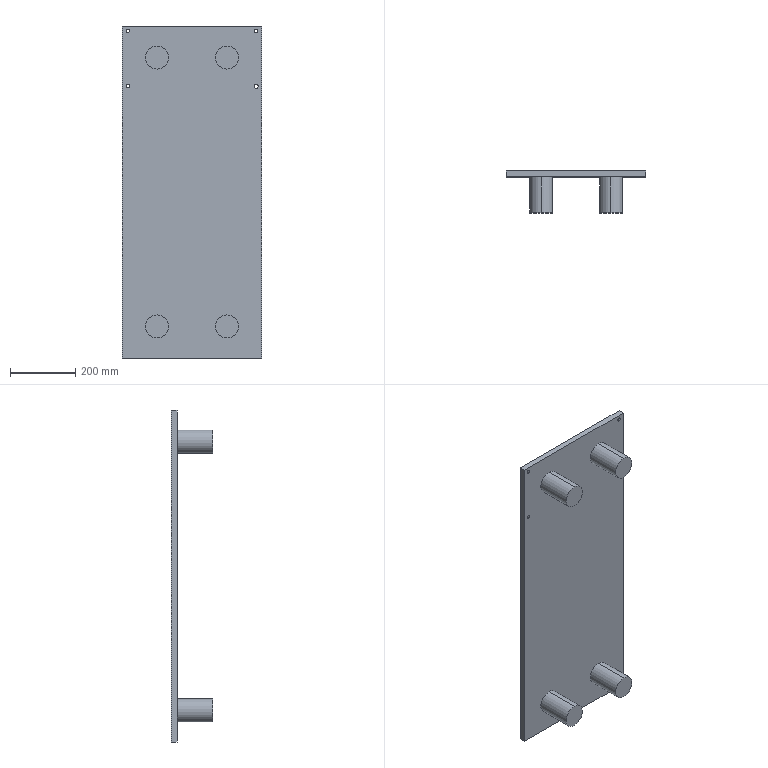Part | SolidWorks | features Extrusion 1, ICE 1 | 1 solid | 26 faces | box 430 x 128 x 1020 mm | volume 9620878 mm3 | cylinder 16 | plane 10 | commonest cylinder face diameters 70.779 x8 10.158 x2 10.702 x2 11 x2 12.721 x2
STEP:
#1=CARTESIAN_POINT('',(96.666,-110.,-468.564));
#2=VERTEX_POINT('',#1);
#3=CARTESIAN_POINT('',(96.666,-110.,-397.785));
#4=VERTEX_POINT('',#3);
#5=CARTESIAN_POINT('',(96.666,-110.,-433.174));
#6=DIRECTION('',(0.,-1.,0.));
#7=DIRECTION('',(0.,0.,1.));
#8=AXIS2_PLACEMENT_3D('',#5,#6,#7);
#9=CIRCLE('',#8,35.39);
#10=EDGE_CURVE('',#2,#4,#9,.T.);
#11=ORIENTED_EDGE('',*,*,#10,.F.);
#12=CARTESIAN_POINT('',(96.666,0.,-468.564));
#13=VERTEX_POINT('',#12);
#14=CARTESIAN_POINT('',(96.666,-110.,-468.564));
#15=DIRECTION('',(0.,1.,0.));
#16=VECTOR('',#15,1000.);
#17=LINE('',#14,#16);
#18=EDGE_CURVE('',#2,#13,#17,.T.);
#19=ORIENTED_EDGE('',*,*,#18,.T.);
#20=CARTESIAN_POINT('',(96.666,0.,-397.785));
#21=VERTEX_POINT('',#20);
#22=CARTESIAN_POINT('',(96.666,0.,-433.174));
#23=DIRECTION('',(0.,-1.,0.));
#24=DIRECTION('',(0.,0.,1.));
#25=AXIS2_PLACEMENT_3D('',#22,#23,#24);
#26=CIRCLE('',#25,35.39);
#27=EDGE_CURVE('',#13,#21,#26,.T.);
#28=ORIENTED_EDGE('',*,*,#27,.T.);
#29=CARTESIAN_POINT('',(96.666,-110.,-397.785));
#30=DIRECTION('',(0.,1.,0.));
#31=VECTOR('',#30,1000.);
#32=LINE('',#29,#31);
#33=EDGE_CURVE('',#4,#21,#32,.T.);
#34=ORIENTED_EDGE('',*,*,#33,.F.);
#35=EDGE_LOOP('',(#11,#19,#28,#34));
#36=FACE_OUTER_BOUND('',#35,.T.);
#37=CARTESIAN_POINT('',(96.666,-110.,-433.174));
#38=DIRECTION('',(0.,1.,0.));
#39=DIRECTION('',(0.,0.,1.));
#40=AXIS2_PLACEMENT_3D('',#37,#38,#39);
#41=CYLINDRICAL_SURFACE('',#40,35.39);
#42=ADVANCED_FACE('',(#36),#41,.T.);
#43=CARTESIAN_POINT('',(-118.27,-110.,-468.564));
#44=VERTEX_POINT('',#43);
#45=CARTESIAN_POINT('',(-118.27,-110.,-397.785));
#46=VERTEX_POINT('',#45);
#47=CARTESIAN_POINT('',(-118.27,-110.,-433.174));
#48=DIRECTION('',(0.,-1.,0.));
#49=DIRECTION('',(0.,0.,-1.));
#50=AXIS2_PLACEMENT_3D('',#47,#48,#49);
#51=CIRCLE('',#50,35.39);
#52=EDGE_CURVE('',#44,#46,#51,.T.);
#53=ORIENTED_EDGE('',*,*,#52,.F.);
#54=CARTESIAN_POINT('',(-118.27,0.,-468.564));
#55=VERTEX_POINT('',#54);
#56=CARTESIAN_POINT('',(-118.27,-110.,-468.564));
#57=DIRECTION('',(0.,1.,0.));
#58=VECTOR('',#57,1000.);
#59=LINE('',#56,#58);
#60=EDGE_CURVE('',#44,#55,#59,.T.);
#61=ORIENTED_EDGE('',*,*,#60,.T.);
#62=CARTESIAN_POINT('',(-118.27,0.,-397.785));
#63=VERTEX_POINT('',#62);
#64=CARTESIAN_POINT('',(-118.27,0.,-433.174));
#65=DIRECTION('',(0.,-1.,0.));
#66=DIRECTION('',(0.,0.,1.));
#67=AXIS2_PLACEMENT_3D('',#64,#65,#66);
#68=CIRCLE('',#67,35.39);
#69=EDGE_CURVE('',#55,#63,#68,.T.);
#70=ORIENTED_EDGE('',*,*,#69,.T.);
#71=CARTESIAN_POINT('',(-118.27,-110.,-397.785));
#72=DIRECTION('',(0.,1.,0.));
#73=VECTOR('',#72,1000.);
#74=LINE('',#71,#73);
#75=EDGE_CURVE('',#46,#63,#74,.T.);
#76=ORIENTED_EDGE('',*,*,#75,.F.);
#77=EDGE_LOOP('',(#53,#61,#70,#76));
#78=FACE_OUTER_BOUND('',#77,.T.);
#79=CARTESIAN_POINT('',(-118.27,-110.,-433.174));
#80=DIRECTION('',(0.,1.,0.));
#81=DIRECTION('',(0.,0.,1.));
#82=AXIS2_PLACEMENT_3D('',#79,#80,#81);
#83=CYLINDRICAL_SURFACE('',#82,35.39);
#84=ADVANCED_FACE('',(#78),#83,.T.);
#85=CARTESIAN_POINT('',(-118.27,-110.,357.683));
#86=VERTEX_POINT('',#85);
#87=CARTESIAN_POINT('',(-118.27,-110.,428.463));
#88=VERTEX_POINT('',#87);
#89=CARTESIAN_POINT('',(-118.27,-110.,393.073));
#90=DIRECTION('',(0.,-1.,0.));
#91=DIRECTION('',(0.,0.,1.));
#92=AXIS2_PLACEMENT_3D('',#89,#90,#91);
#93=CIRCLE('',#92,35.39);
#94=EDGE_CURVE('',#86,#88,#93,.T.);
#95=ORIENTED_EDGE('',*,*,#94,.F.);
#96=CARTESIAN_POINT('',(-118.27,0.,357.683));
#97=VERTEX_POINT('',#96);
#98=CARTESIAN_POINT('',(-118.27,-110.,357.683));
#99=DIRECTION('',(0.,1.,0.));
#100=VECTOR('',#99,1000.);
#101=LINE('',#98,#100);
#102=EDGE_CURVE('',#86,#97,#101,.T.);
#103=ORIENTED_EDGE('',*,*,#102,.T.);
#104=CARTESIAN_POINT('',(-118.27,0.,428.463));
#105=VERTEX_POINT('',#104);
#106=CARTESIAN_POINT('',(-118.27,0.,393.073));
#107=DIRECTION('',(0.,-1.,0.));
#108=DIRECTION('',(0.,0.,1.));
#109=AXIS2_PLACEMENT_3D('',#106,#107,#108);
#110=CIRCLE('',#109,35.39);
#111=EDGE_CURVE('',#97,#105,#110,.T.);
#112=ORIENTED_EDGE('',*,*,#111,.T.);
#113=CARTESIAN_POINT('',(-118.27,-110.,428.463));
#114=DIRECTION('',(0.,1.,0.));
#115=VECTOR('',#114,1000.);
#116=LINE('',#113,#115);
#117=EDGE_CURVE('',#88,#105,#116,.T.);
#118=ORIENTED_EDGE('',*,*,#117,.F.);
#119=EDGE_LOOP('',(#95,#103,#112,#118));
#120=FACE_OUTER_BOUND('',#119,.T.);
#121=CARTESIAN_POINT('',(-118.27,-110.,393.073));
#122=DIRECTION('',(0.,1.,0.));
#123=DIRECTION('',(0.,0.,1.));
#124=AXIS2_PLACEMENT_3D('',#121,#122,#123);
#125=CYLINDRICAL_SURFACE('',#124,35.39);
#126=ADVANCED_FACE('',(#120),#125,.T.);
#127=CARTESIAN_POINT('',(96.666,-110.,357.683));
#128=VERTEX_POINT('',#127);
#129=CARTESIAN_POINT('',(96.666,-110.,428.463));
#130=VERTEX_POINT('',#129);
#131=CARTESIAN_POINT('',(96.666,-110.,393.073));
#132=DIRECTION('',(0.,-1.,0.));
#133=DIRECTION('',(0.,0.,-1.));
#134=AXIS2_PLACEMENT_3D('',#131,#132,#133);
#135=CIRCLE('',#134,35.39);
#136=EDGE_CURVE('',#128,#130,#135,.T.);
#137=ORIENTED_EDGE('',*,*,#136,.F.);
#138=CARTESIAN_POINT('',(96.666,0.,357.683));
#139=VERTEX_POINT('',#138);
#140=CARTESIAN_POINT('',(96.666,-110.,357.683));
#141=DIRECTION('',(0.,1.,0.));
#142=VECTOR('',#141,1000.);
#143=LINE('',#140,#142);
#144=EDGE_CURVE('',#128,#139,#143,.T.);
#145=ORIENTED_EDGE('',*,*,#144,.T.);
#146=CARTESIAN_POINT('',(96.666,0.,428.463));
#147=VERTEX_POINT('',#146);
#148=CARTESIAN_POINT('',(96.666,0.,393.073));
#149=DIRECTION('',(0.,-1.,0.));
#150=DIRECTION('',(0.,0.,1.));
#151=AXIS2_PLACEMENT_3D('',#148,#149,#150);
#152=CIRCLE('',#151,35.39);
#153=EDGE_CURVE('',#139,#147,#152,.T.);
#154=ORIENTED_EDGE('',*,*,#153,.T.);
#155=CARTESIAN_POINT('',(96.666,-110.,428.463));
#156=DIRECTION('',(0.,1.,0.));
#157=VECTOR('',#156,1000.);
#158=LINE('',#155,#157);
#159=EDGE_CURVE('',#130,#147,#158,.T.);
#160=ORIENTED_EDGE('',*,*,#159,.F.);
#161=EDGE_LOOP('',(#137,#145,#154,#160));
#162=FACE_OUTER_BOUND('',#161,.T.);
#163=CARTESIAN_POINT('',(96.666,-110.,393.073));
#164=DIRECTION('',(0.,1.,0.));
#165=DIRECTION('',(0.,0.,1.));
#166=AXIS2_PLACEMENT_3D('',#163,#164,#165);
#167=CYLINDRICAL_SURFACE('',#166,35.39);
#168=ADVANCED_FACE('',(#162),#167,.T.);
#169=CARTESIAN_POINT('',(-207.802,18.,469.994));
#170=VERTEX_POINT('',#169);
#171=CARTESIAN_POINT('',(-207.802,18.,480.153));
#172=VERTEX_POINT('',#171);
#173=CARTESIAN_POINT('',(-207.802,18.,475.073));
#174=DIRECTION('',(0.,1.,0.));
#175=DIRECTION('',(0.,0.,1.));
#176=AXIS2_PLACEMENT_3D('',#173,#174,#175);
#177=CIRCLE('',#176,5.079);
#178=EDGE_CURVE('',#170,#172,#177,.T.);
#179=ORIENTED_EDGE('',*,*,#178,.T.);
#180=CARTESIAN_POINT('',(-207.802,0.,480.153));
#181=VERTEX_POINT('',#180);
#182=CARTESIAN_POINT('',(-207.802,18.,480.153));
#183=DIRECTION('',(0.,-1.,0.));
#184=VECTOR('',#183,1000.);
#185=LINE('',#182,#184);
#186=EDGE_CURVE('',#172,#181,#185,.T.);
#187=ORIENTED_EDGE('',*,*,#186,.T.);
#188=CARTESIAN_POINT('',(-207.802,0.,469.994));
#189=VERTEX_POINT('',#188);
#190=CARTESIAN_POINT('',(-207.802,0.,475.073));
#191=DIRECTION('',(0.,1.,0.));
#192=DIRECTION('',(0.,0.,1.));
#193=AXIS2_PLACEMENT_3D('',#190,#191,#192);
#194=CIRCLE('',#193,5.079);
#195=EDGE_CURVE('',#189,#181,#194,.T.);
#196=ORIENTED_EDGE('',*,*,#195,.F.);
#197=CARTESIAN_POINT('',(-207.802,18.,469.994));
#198=DIRECTION('',(0.,-1.,0.));
#199=VECTOR('',#198,1000.);
#200=LINE('',#197,#199);
#201=EDGE_CURVE('',#170,#189,#200,.T.);
#202=ORIENTED_EDGE('',*,*,#201,.F.);
#203=EDGE_LOOP('',(#179,#187,#196,#202));
#204=FACE_OUTER_BOUND('',#203,.T.);
#205=CARTESIAN_POINT('',(-207.802,18.,475.073));
#206=DIRECTION('',(0.,-1.,0.));
#207=DIRECTION('',(0.,0.,-1.));
#208=AXIS2_PLACEMENT_3D('',#205,#206,#207);
#209=CYLINDRICAL_SURFACE('',#208,5.079);
#210=ADVANCED_FACE('',(#204),#209,.F.);
#211=CARTESIAN_POINT('',(-207.802,18.,299.722));
#212=VERTEX_POINT('',#211);
#213=CARTESIAN_POINT('',(-207.802,18.,310.425));
#214=VERTEX_POINT('',#213);
#215=CARTESIAN_POINT('',(-207.802,18.,305.073));
#216=DIRECTION('',(0.,1.,0.));
#217=DIRECTION('',(0.,0.,1.));
#218=AXIS2_PLACEMENT_3D('',#215,#216,#217);
#219=CIRCLE('',#218,5.351);
#220=EDGE_CURVE('',#212,#214,#219,.T.);
#221=ORIENTED_EDGE('',*,*,#220,.T.);
#222=CARTESIAN_POINT('',(-207.802,0.,310.425));
#223=VERTEX_POINT('',#222);
#224=CARTESIAN_POINT('',(-207.802,18.,310.425));
#225=DIRECTION('',(0.,-1.,0.));
#226=VECTOR('',#225,1000.);
#227=LINE('',#224,#226);
#228=EDGE_CURVE('',#214,#223,#227,.T.);
#229=ORIENTED_EDGE('',*,*,#228,.T.);
#230=CARTESIAN_POINT('',(-207.802,0.,299.722));
#231=VERTEX_POINT('',#230);
#232=CARTESIAN_POINT('',(-207.802,0.,305.073));
#233=DIRECTION('',(0.,1.,0.));
#234=DIRECTION('',(0.,0.,1.));
#235=AXIS2_PLACEMENT_3D('',#232,#233,#234);
#236=CIRCLE('',#235,5.351);
#237=EDGE_CURVE('',#231,#223,#236,.T.);
#238=ORIENTED_EDGE('',*,*,#237,.F.);
#239=CARTESIAN_POINT('',(-207.802,18.,299.722));
#240=DIRECTION('',(0.,-1.,0.));
#241=VECTOR('',#240,1000.);
#242=LINE('',#239,#241);
#243=EDGE_CURVE('',#212,#231,#242,.T.);
#244=ORIENTED_EDGE('',*,*,#243,.F.);
#245=EDGE_LOOP('',(#221,#229,#238,#244));
#246=FACE_OUTER_BOUND('',#245,.T.);
#247=CARTESIAN_POINT('',(-207.802,18.,305.073));
#248=DIRECTION('',(0.,-1.,0.));
#249=DIRECTION('',(0.,0.,-1.));
#250=AXIS2_PLACEMENT_3D('',#247,#248,#249);
#251=CYLINDRICAL_SURFACE('',#250,5.351);
#252=ADVANCED_FACE('',(#246),#251,.F.);
#253=CARTESIAN_POINT('',(186.198,18.,298.713));
#254=VERTEX_POINT('',#253);
#255=CARTESIAN_POINT('',(186.198,18.,311.434));
#256=VERTEX_POINT('',#255);
#257=CARTESIAN_POINT('',(186.198,18.,305.073));
#258=DIRECTION('',(0.,1.,0.));
#259=DIRECTION('',(0.,0.,1.));
#260=AXIS2_PLACEMENT_3D('',#257,#258,#259);
#261=CIRCLE('',#260,6.36);
#262=EDGE_CURVE('',#254,#256,#261,.T.);
#263=ORIENTED_EDGE('',*,*,#262,.T.);
#264=CARTESIAN_POINT('',(186.198,0.,311.434));
#265=VERTEX_POINT('',#264);
#266=CARTESIAN_POINT('',(186.198,18.,311.434));
#267=DIRECTION('',(0.,-1.,0.));
#268=VECTOR('',#267,1000.);
#269=LINE('',#266,#268);
#270=EDGE_CURVE('',#256,#265,#269,.T.);
#271=ORIENTED_EDGE('',*,*,#270,.T.);
#272=CARTESIAN_POINT('',(186.198,0.,298.713));
#273=VERTEX_POINT('',#272);
#274=CARTESIAN_POINT('',(186.198,0.,305.073));
#275=DIRECTION('',(0.,1.,0.));
#276=DIRECTION('',(0.,0.,1.));
#277=AXIS2_PLACEMENT_3D('',#274,#275,#276);
#278=CIRCLE('',#277,6.36);
#279=EDGE_CURVE('',#273,#265,#278,.T.);
#280=ORIENTED_EDGE('',*,*,#279,.F.);
#281=CARTESIAN_POINT('',(186.198,18.,298.713));
#282=DIRECTION('',(0.,-1.,0.));
#283=VECTOR('',#282,1000.);
#284=LINE('',#281,#283);
#285=EDGE_CURVE('',#254,#273,#284,.T.);
#286=ORIENTED_EDGE('',*,*,#285,.F.);
#287=EDGE_LOOP('',(#263,#271,#280,#286));
#288=FACE_OUTER_BOUND('',#287,.T.);
#289=CARTESIAN_POINT('',(186.198,18.,305.073));
#290=DIRECTION('',(0.,-1.,0.));
#291=DIRECTION('',(0.,0.,-1.));
#292=AXIS2_PLACEMENT_3D('',#289,#290,#291);
#293=CYLINDRICAL_SURFACE('',#292,6.36);
#294=ADVANCED_FACE('',(#288),#293,.F.);
#295=CARTESIAN_POINT('',(186.198,18.,469.573));
#296=VERTEX_POINT('',#295);
#297=CARTESIAN_POINT('',(186.198,18.,480.573));
#298=VERTEX_POINT('',#297);
#299=CARTESIAN_POINT('',(186.198,18.,475.073));
#300=DIRECTION('',(0.,1.,0.));
#301=DIRECTION('',(0.,0.,1.));
#302=AXIS2_PLACEMENT_3D('',#299,#300,#301);
#303=CIRCLE('',#302,5.5);
#304=EDGE_CURVE('',#296,#298,#303,.T.);
#305=ORIENTED_EDGE('',*,*,#304,.T.);
#306=CARTESIAN_POINT('',(186.198,0.,480.573));
#307=VERTEX_POINT('',#306);
#308=CARTESIAN_POINT('',(186.198,18.,480.573));
#309=DIRECTION('',(0.,-1.,0.));
#310=VECTOR('',#309,1000.);
#311=LINE('',#308,#310);
#312=EDGE_CURVE('',#298,#307,#311,.T.);
#313=ORIENTED_EDGE('',*,*,#312,.T.);
#314=CARTESIAN_POINT('',(186.198,0.,469.573));
#315=VERTEX_POINT('',#314);
#316=CARTESIAN_POINT('',(186.198,0.,475.073));
#317=DIRECTION('',(0.,1.,0.));
#318=DIRECTION('',(0.,0.,1.));
#319=AXIS2_PLACEMENT_3D('',#316,#317,#318);
#320=CIRCLE('',#319,5.5);
#321=EDGE_CURVE('',#315,#307,#320,.T.);
#322=ORIENTED_EDGE('',*,*,#321,.F.);
#323=CARTESIAN_POINT('',(186.198,18.,469.573));
#324=DIRECTION('',(0.,-1.,0.));
#325=VECTOR('',#324,1000.);
#326=LINE('',#323,#325);
#327=EDGE_CURVE('',#296,#315,#326,.T.);
#328=ORIENTED_EDGE('',*,*,#327,.F.);
#329=EDGE_LOOP('',(#305,#313,#322,#328));
#330=FACE_OUTER_BOUND('',#329,.T.);
#331=CARTESIAN_POINT('',(186.198,18.,475.073));
#332=DIRECTION('',(0.,-1.,0.));
#333=DIRECTION('',(0.,0.,-1.));
#334=AXIS2_PLACEMENT_3D('',#331,#332,#333);
#335=CYLINDRICAL_SURFACE('',#334,5.5);
#336=ADVANCED_FACE('',(#330),#335,.F.);
#337=ORIENTED_EDGE('',*,*,#220,.F.);
#338=CARTESIAN_POINT('',(-207.802,18.,305.073));
#339=DIRECTION('',(0.,1.,0.));
#340=DIRECTION('',(0.,0.,1.));
#341=AXIS2_PLACEMENT_3D('',#338,#339,#340);
#342=CIRCLE('',#341,5.351);
#343=EDGE_CURVE('',#214,#212,#342,.T.);
#344=ORIENTED_EDGE('',*,*,#343,.F.);
#345=EDGE_LOOP('',(#337,#344));
#346=FACE_BOUND('',#345,.T.);
#347=ORIENTED_EDGE('',*,*,#304,.F.);
#348=CARTESIAN_POINT('',(186.198,18.,475.073));
#349=DIRECTION('',(0.,1.,0.));
#350=DIRECTION('',(0.,0.,1.));
#351=AXIS2_PLACEMENT_3D('',#348,#349,#350);
#352=CIRCLE('',#351,5.5);
#353=EDGE_CURVE('',#298,#296,#352,.T.);
#354=ORIENTED_EDGE('',*,*,#353,.F.);
#355=EDGE_LOOP('',(#347,#354));
#356=FACE_BOUND('',#355,.T.);
#357=CARTESIAN_POINT('',(204.198,18.,490.073));
#358=VERTEX_POINT('',#357);
#359=CARTESIAN_POINT('',(204.198,18.,-530.175));
#360=VERTEX_POINT('',#359);
#361=CARTESIAN_POINT('',(204.198,18.,490.073));
#362=DIRECTION('',(0.,0.,-1.));
#363=VECTOR('',#362,1000.);
#364=LINE('',#361,#363);
#365=EDGE_CURVE('',#358,#360,#364,.T.);
#366=ORIENTED_EDGE('',*,*,#365,.T.);
#367=CARTESIAN_POINT('',(-225.802,18.,-530.175));
#368=VERTEX_POINT('',#367);
#369=CARTESIAN_POINT('',(204.198,18.,-530.175));
#370=DIRECTION('',(-1.,0.,0.));
#371=VECTOR('',#370,1000.);
#372=LINE('',#369,#371);
#373=EDGE_CURVE('',#360,#368,#372,.T.);
#374=ORIENTED_EDGE('',*,*,#373,.T.);
#375=CARTESIAN_POINT('',(-225.802,18.,490.073));
#376=VERTEX_POINT('',#375);
#377=CARTESIAN_POINT('',(-225.802,18.,290.073));
#378=DIRECTION('',(0.,0.,1.));
#379=VECTOR('',#378,1000.);
#380=LINE('',#377,#379);
#381=EDGE_CURVE('',#368,#376,#380,.T.);
#382=ORIENTED_EDGE('',*,*,#381,.T.);
#383=CARTESIAN_POINT('',(204.198,18.,490.073));
#384=DIRECTION('',(1.,0.,0.));
#385=VECTOR('',#384,1000.);
#386=LINE('',#383,#385);
#387=EDGE_CURVE('',#376,#358,#386,.T.);
#388=ORIENTED_EDGE('',*,*,#387,.T.);
#389=EDGE_LOOP('',(#366,#374,#382,#388));
#390=FACE_OUTER_BOUND('',#389,.T.);
#391=ORIENTED_EDGE('',*,*,#262,.F.);
#392=CARTESIAN_POINT('',(186.198,18.,305.073));
#393=DIRECTION('',(0.,1.,0.));
#394=DIRECTION('',(0.,0.,1.));
#395=AXIS2_PLACEMENT_3D('',#392,#393,#394);
#396=CIRCLE('',#395,6.36);
#397=EDGE_CURVE('',#256,#254,#396,.T.);
#398=ORIENTED_EDGE('',*,*,#397,.F.);
#399=EDGE_LOOP('',(#391,#398));
#400=FACE_BOUND('',#399,.T.);
#401=ORIENTED_EDGE('',*,*,#178,.F.);
#402=CARTESIAN_POINT('',(-207.802,18.,475.073));
#403=DIRECTION('',(0.,1.,0.));
#404=DIRECTION('',(0.,0.,1.));
#405=AXIS2_PLACEMENT_3D('',#402,#403,#404);
#406=CIRCLE('',#405,5.079);
#407=EDGE_CURVE('',#172,#170,#406,.T.);
#408=ORIENTED_EDGE('',*,*,#407,.F.);
#409=EDGE_LOOP('',(#401,#408));
#410=FACE_BOUND('',#409,.T.);
#411=CARTESIAN_POINT('',(0.,18.,0.));
#412=DIRECTION('',(0.,1.,0.));
#413=DIRECTION('',(0.,0.,1.));
#414=AXIS2_PLACEMENT_3D('',#411,#412,#413);
#415=PLANE('',#414);
#416=ADVANCED_FACE('',(#346,#356,#390,#400,#410),#415,.T.);
#417=CARTESIAN_POINT('',(96.666,0.,-433.174));
#418=DIRECTION('',(0.,-1.,0.));
#419=DIRECTION('',(0.,0.,1.));
#420=AXIS2_PLACEMENT_3D('',#417,#418,#419);
#421=CIRCLE('',#420,35.39);
#422=EDGE_CURVE('',#21,#13,#421,.T.);
#423=ORIENTED_EDGE('',*,*,#422,.F.);
#424=ORIENTED_EDGE('',*,*,#27,.F.);
#425=EDGE_LOOP('',(#423,#424));
#426=FACE_BOUND('',#425,.T.);
#427=CARTESIAN_POINT('',(-118.27,0.,-433.174));
#428=DIRECTION('',(0.,-1.,0.));
#429=DIRECTION('',(0.,0.,1.));
#430=AXIS2_PLACEMENT_3D('',#427,#428,#429);
#431=CIRCLE('',#430,35.39);
#432=EDGE_CURVE('',#63,#55,#431,.T.);
#433=ORIENTED_EDGE('',*,*,#432,.F.);
#434=ORIENTED_EDGE('',*,*,#69,.F.);
#435=EDGE_LOOP('',(#433,#434));
#436=FACE_BOUND('',#435,.T.);
#437=CARTESIAN_POINT('',(-118.27,0.,393.073));
#438=DIRECTION('',(0.,-1.,0.));
#439=DIRECTION('',(0.,0.,1.));
#440=AXIS2_PLACEMENT_3D('',#437,#438,#439);
#441=CIRCLE('',#440,35.39);
#442=EDGE_CURVE('',#105,#97,#441,.T.);
#443=ORIENTED_EDGE('',*,*,#442,.F.);
#444=ORIENTED_EDGE('',*,*,#111,.F.);
#445=EDGE_LOOP('',(#443,#444));
#446=FACE_BOUND('',#445,.T.);
#447=CARTESIAN_POINT('',(96.666,0.,393.073));
#448=DIRECTION('',(0.,-1.,0.));
#449=DIRECTION('',(0.,0.,1.));
#450=AXIS2_PLACEMENT_3D('',#447,#448,#449);
#451=CIRCLE('',#450,35.39);
#452=EDGE_CURVE('',#147,#139,#451,.T.);
#453=ORIENTED_EDGE('',*,*,#452,.F.);
#454=ORIENTED_EDGE('',*,*,#153,.F.);
#455=EDGE_LOOP('',(#453,#454));
#456=FACE_BOUND('',#455,.T.);
#457=CARTESIAN_POINT('',(204.198,0.,490.073));
#458=VERTEX_POINT('',#457);
#459=CARTESIAN_POINT('',(204.198,0.,-530.175));
#460=VERTEX_POINT('',#459);
#461=CARTESIAN_POINT('',(204.198,0.,490.073));
#462=DIRECTION('',(0.,0.,-1.));
#463=VECTOR('',#462,1000.);
#464=LINE('',#461,#463);
#465=EDGE_CURVE('',#458,#460,#464,.T.);
#466=ORIENTED_EDGE('',*,*,#465,.F.);
#467=CARTESIAN_POINT('',(-225.802,0.,490.073));
#468=VERTEX_POINT('',#467);
#469=CARTESIAN_POINT('',(204.198,0.,490.073));
#470=DIRECTION('',(1.,0.,0.));
#471=VECTOR('',#470,1000.);
#472=LINE('',#469,#471);
#473=EDGE_CURVE('',#468,#458,#472,.T.);
#474=ORIENTED_EDGE('',*,*,#473,.F.);
#475=CARTESIAN_POINT('',(-225.802,0.,-530.175));
#476=VERTEX_POINT('',#475);
#477=CARTESIAN_POINT('',(-225.802,0.,490.073));
#478=DIRECTION('',(0.,0.,1.));
#479=VECTOR('',#478,1000.);
#480=LINE('',#477,#479);
#481=EDGE_CURVE('',#476,#468,#480,.T.);
#482=ORIENTED_EDGE('',*,*,#481,.F.);
#483=CARTESIAN_POINT('',(204.198,0.,-530.175));
#484=DIRECTION('',(-1.,0.,0.));
#485=VECTOR('',#484,1000.);
#486=LINE('',#483,#485);
#487=EDGE_CURVE('',#460,#476,#486,.T.);
#488=ORIENTED_EDGE('',*,*,#487,.F.);
#489=EDGE_LOOP('',(#466,#474,#482,#488));
#490=FACE_OUTER_BOUND('',#489,.T.);
#491=ORIENTED_EDGE('',*,*,#321,.T.);
#492=CARTESIAN_POINT('',(186.198,0.,475.073));
#493=DIRECTION('',(0.,1.,0.));
#494=DIRECTION('',(0.,0.,1.));
#495=AXIS2_PLACEMENT_3D('',#492,#493,#494);
#496=CIRCLE('',#495,5.5);
#497=EDGE_CURVE('',#307,#315,#496,.T.);
#498=ORIENTED_EDGE('',*,*,#497,.T.);
#499=EDGE_LOOP('',(#491,#498));
#500=FACE_BOUND('',#499,.T.);
#501=ORIENTED_EDGE('',*,*,#279,.T.);
#502=CARTESIAN_POINT('',(186.198,0.,305.073));
#503=DIRECTION('',(0.,1.,0.));
#504=DIRECTION('',(0.,0.,1.));
#505=AXIS2_PLACEMENT_3D('',#502,#503,#504);
#506=CIRCLE('',#505,6.36);
#507=EDGE_CURVE('',#265,#273,#506,.T.);
#508=ORIENTED_EDGE('',*,*,#507,.T.);
#509=EDGE_LOOP('',(#501,#508));
#510=FACE_BOUND('',#509,.T.);
#511=ORIENTED_EDGE('',*,*,#237,.T.);
#512=CARTESIAN_POINT('',(-207.802,0.,305.073));
#513=DIRECTION('',(0.,1.,0.));
#514=DIRECTION('',(0.,0.,1.));
#515=AXIS2_PLACEMENT_3D('',#512,#513,#514);
#516=CIRCLE('',#515,5.351);
#517=EDGE_CURVE('',#223,#231,#516,.T.);
#518=ORIENTED_EDGE('',*,*,#517,.T.);
#519=EDGE_LOOP('',(#511,#518));
#520=FACE_BOUND('',#519,.T.);
#521=ORIENTED_EDGE('',*,*,#195,.T.);
#522=CARTESIAN_POINT('',(-207.802,0.,475.073));
#523=DIRECTION('',(0.,1.,0.));
#524=DIRECTION('',(0.,0.,1.));
#525=AXIS2_PLACEMENT_3D('',#522,#523,#524);
#526=CIRCLE('',#525,5.079);
#527=EDGE_CURVE('',#181,#189,#526,.T.);
#528=ORIENTED_EDGE('',*,*,#527,.T.);
#529=EDGE_LOOP('',(#521,#528));
#530=FACE_BOUND('',#529,.T.);
#531=CARTESIAN_POINT('',(0.,0.,0.));
#532=DIRECTION('',(0.,1.,0.));
#533=DIRECTION('',(0.,0.,1.));
#534=AXIS2_PLACEMENT_3D('',#531,#532,#533);
#535=PLANE('',#534);
#536=ADVANCED_FACE('',(#426,#436,#446,#456,#490,#500,#510,#520,#530),#535,.F.);
#537=ORIENTED_EDGE('',*,*,#465,.T.);
#538=CARTESIAN_POINT('',(204.198,18.,-530.175));
#539=DIRECTION('',(0.,-1.,0.));
#540=VECTOR('',#539,1000.);
#541=LINE('',#538,#540);
#542=EDGE_CURVE('',#360,#460,#541,.T.);
#543=ORIENTED_EDGE('',*,*,#542,.F.);
#544=ORIENTED_EDGE('',*,*,#365,.F.);
#545=CARTESIAN_POINT('',(204.198,18.,490.073));
#546=DIRECTION('',(0.,-1.,0.));
#547=VECTOR('',#546,1000.);
#548=LINE('',#545,#547);
#549=EDGE_CURVE('',#358,#458,#548,.T.);
#550=ORIENTED_EDGE('',*,*,#549,.T.);
#551=EDGE_LOOP('',(#537,#543,#544,#550));
#552=FACE_OUTER_BOUND('',#551,.T.);
#553=CARTESIAN_POINT('',(204.198,18.,490.073));
#554=DIRECTION('',(-1.,0.,0.));
#555=DIRECTION('',(0.,0.,1.));
#556=AXIS2_PLACEMENT_3D('',#553,#554,#555);
#557=PLANE('',#556);
#558=ADVANCED_FACE('',(#552),#557,.F.);
#559=ORIENTED_EDGE('',*,*,#487,.T.);
#560=CARTESIAN_POINT('',(-225.802,18.,-530.175));
#561=DIRECTION('',(0.,-1.,0.));
#562=VECTOR('',#561,1000.);
#563=LINE('',#560,#562);
#564=EDGE_CURVE('',#368,#476,#563,.T.);
#565=ORIENTED_EDGE('',*,*,#564,.F.);
#566=ORIENTED_EDGE('',*,*,#373,.F.);
#567=ORIENTED_EDGE('',*,*,#542,.T.);
#568=EDGE_LOOP('',(#559,#565,#566,#567));
#569=FACE_OUTER_BOUND('',#568,.T.);
#570=CARTESIAN_POINT('',(204.198,18.,-530.175));
#571=DIRECTION('',(0.,0.,1.));
#572=DIRECTION('',(1.,0.,0.));
#573=AXIS2_PLACEMENT_3D('',#570,#571,#572);
#574=PLANE('',#573);
#575=ADVANCED_FACE('',(#569),#574,.F.);
#576=ORIENTED_EDGE('',*,*,#481,.T.);
#577=CARTESIAN_POINT('',(-225.802,18.,490.073));
#578=DIRECTION('',(0.,-1.,0.));
#579=VECTOR('',#578,1000.);
#580=LINE('',#577,#579);
#581=EDGE_CURVE('',#376,#468,#580,.T.);
#582=ORIENTED_EDGE('',*,*,#581,.F.);
#583=ORIENTED_EDGE('',*,*,#381,.F.);
#584=ORIENTED_EDGE('',*,*,#564,.T.);
#585=EDGE_LOOP('',(#576,#582,#583,#584));
#586=FACE_OUTER_BOUND('',#585,.T.);
#587=CARTESIAN_POINT('',(-225.802,18.,490.073));
#588=DIRECTION('',(1.,0.,0.));
#589=DIRECTION('',(0.,0.,-1.));
#590=AXIS2_PLACEMENT_3D('',#587,#588,#589);
#591=PLANE('',#590);
#592=ADVANCED_FACE('',(#586),#591,.F.);
#593=ORIENTED_EDGE('',*,*,#473,.T.);
#594=ORIENTED_EDGE('',*,*,#549,.F.);
#595=ORIENTED_EDGE('',*,*,#387,.F.);
#596=ORIENTED_EDGE('',*,*,#581,.T.);
#597=EDGE_LOOP('',(#593,#594,#595,#596));
#598=FACE_OUTER_BOUND('',#597,.T.);
#599=CARTESIAN_POINT('',(204.198,18.,490.073));
#600=DIRECTION('',(0.,0.,-1.));
#601=DIRECTION('',(-1.,0.,0.));
#602=AXIS2_PLACEMENT_3D('',#599,#600,#601);
#603=PLANE('',#602);
#604=ADVANCED_FACE('',(#598),#603,.F.);
#605=ORIENTED_EDGE('',*,*,#312,.F.);
#606=ORIENTED_EDGE('',*,*,#353,.T.);
#607=ORIENTED_EDGE('',*,*,#327,.T.);
#608=ORIENTED_EDGE('',*,*,#497,.F.);
#609=EDGE_LOOP('',(#605,#606,#607,#608));
#610=FACE_OUTER_BOUND('',#609,.T.);
#611=CARTESIAN_POINT('',(186.198,18.,475.073));
#612=DIRECTION('',(0.,-1.,0.));
#613=DIRECTION('',(0.,0.,-1.));
#614=AXIS2_PLACEMENT_3D('',#611,#612,#613);
#615=CYLINDRICAL_SURFACE('',#614,5.5);
#616=ADVANCED_FACE('',(#610),#615,.F.);
#617=ORIENTED_EDGE('',*,*,#270,.F.);
#618=ORIENTED_EDGE('',*,*,#397,.T.);
#619=ORIENTED_EDGE('',*,*,#285,.T.);
#620=ORIENTED_EDGE('',*,*,#507,.F.);
#621=EDGE_LOOP('',(#617,#618,#619,#620));
#622=FACE_OUTER_BOUND('',#621,.T.);
#623=CARTESIAN_POINT('',(186.198,18.,305.073));
#624=DIRECTION('',(0.,-1.,0.));
#625=DIRECTION('',(0.,0.,-1.));
#626=AXIS2_PLACEMENT_3D('',#623,#624,#625);
#627=CYLINDRICAL_SURFACE('',#626,6.36);
#628=ADVANCED_FACE('',(#622),#627,.F.);
#629=ORIENTED_EDGE('',*,*,#228,.F.);
#630=ORIENTED_EDGE('',*,*,#343,.T.);
#631=ORIENTED_EDGE('',*,*,#243,.T.);
#632=ORIENTED_EDGE('',*,*,#517,.F.);
#633=EDGE_LOOP('',(#629,#630,#631,#632));
#634=FACE_OUTER_BOUND('',#633,.T.);
#635=CARTESIAN_POINT('',(-207.802,18.,305.073));
#636=DIRECTION('',(0.,-1.,0.));
#637=DIRECTION('',(0.,0.,-1.));
#638=AXIS2_PLACEMENT_3D('',#635,#636,#637);
#639=CYLINDRICAL_SURFACE('',#638,5.351);
#640=ADVANCED_FACE('',(#634),#639,.F.);
#641=ORIENTED_EDGE('',*,*,#186,.F.);
#642=ORIENTED_EDGE('',*,*,#407,.T.);
#643=ORIENTED_EDGE('',*,*,#201,.T.);
#644=ORIENTED_EDGE('',*,*,#527,.F.);
#645=EDGE_LOOP('',(#641,#642,#643,#644));
#646=FACE_OUTER_BOUND('',#645,.T.);
#647=CARTESIAN_POINT('',(-207.802,18.,475.073));
#648=DIRECTION('',(0.,-1.,0.));
#649=DIRECTION('',(0.,0.,-1.));
#650=AXIS2_PLACEMENT_3D('',#647,#648,#649);
#651=CYLINDRICAL_SURFACE('',#650,5.079);
#652=ADVANCED_FACE('',(#646),#651,.F.);
#653=ORIENTED_EDGE('',*,*,#144,.F.);
#654=CARTESIAN_POINT('',(96.666,-110.,393.073));
#655=DIRECTION('',(0.,-1.,0.));
#656=DIRECTION('',(0.,0.,-1.));
#657=AXIS2_PLACEMENT_3D('',#654,#655,#656);
#658=CIRCLE('',#657,35.39);
#659=EDGE_CURVE('',#130,#128,#658,.T.);
#660=ORIENTED_EDGE('',*,*,#659,.F.);
#661=ORIENTED_EDGE('',*,*,#159,.T.);
#662=ORIENTED_EDGE('',*,*,#452,.T.);
#663=EDGE_LOOP('',(#653,#660,#661,#662));
#664=FACE_OUTER_BOUND('',#663,.T.);
#665=CARTESIAN_POINT('',(96.666,-110.,393.073));
#666=DIRECTION('',(0.,1.,0.));
#667=DIRECTION('',(0.,0.,1.));
#668=AXIS2_PLACEMENT_3D('',#665,#666,#667);
#669=CYLINDRICAL_SURFACE('',#668,35.39);
#670=ADVANCED_FACE('',(#664),#669,.T.);
#671=ORIENTED_EDGE('',*,*,#659,.T.);
#672=ORIENTED_EDGE('',*,*,#136,.T.);
#673=EDGE_LOOP('',(#671,#672));
#674=FACE_OUTER_BOUND('',#673,.T.);
#675=CARTESIAN_POINT('',(96.666,-110.,393.073));
#676=DIRECTION('',(0.,-1.,0.));
#677=DIRECTION('',(0.,0.,-1.));
#678=AXIS2_PLACEMENT_3D('',#675,#676,#677);
#679=PLANE('',#678);
#680=ADVANCED_FACE('',(#674),#679,.T.);
#681=ORIENTED_EDGE('',*,*,#102,.F.);
#682=CARTESIAN_POINT('',(-118.27,-110.,393.073));
#683=DIRECTION('',(0.,-1.,0.));
#684=DIRECTION('',(0.,0.,1.));
#685=AXIS2_PLACEMENT_3D('',#682,#683,#684);
#686=CIRCLE('',#685,35.39);
#687=EDGE_CURVE('',#88,#86,#686,.T.);
#688=ORIENTED_EDGE('',*,*,#687,.F.);
#689=ORIENTED_EDGE('',*,*,#117,.T.);
#690=ORIENTED_EDGE('',*,*,#442,.T.);
#691=EDGE_LOOP('',(#681,#688,#689,#690));
#692=FACE_OUTER_BOUND('',#691,.T.);
#693=CARTESIAN_POINT('',(-118.27,-110.,393.073));
#694=DIRECTION('',(0.,1.,0.));
#695=DIRECTION('',(0.,0.,1.));
#696=AXIS2_PLACEMENT_3D('',#693,#694,#695);
#697=CYLINDRICAL_SURFACE('',#696,35.39);
#698=ADVANCED_FACE('',(#692),#697,.T.);
#699=ORIENTED_EDGE('',*,*,#687,.T.);
#700=ORIENTED_EDGE('',*,*,#94,.T.);
#701=EDGE_LOOP('',(#699,#700));
#702=FACE_OUTER_BOUND('',#701,.T.);
#703=CARTESIAN_POINT('',(-118.27,-110.,393.073));
#704=DIRECTION('',(0.,1.,0.));
#705=DIRECTION('',(0.,0.,1.));
#706=AXIS2_PLACEMENT_3D('',#703,#704,#705);
#707=PLANE('',#706);
#708=ADVANCED_FACE('',(#702),#707,.F.);
#709=ORIENTED_EDGE('',*,*,#60,.F.);
#710=CARTESIAN_POINT('',(-118.27,-110.,-433.174));
#711=DIRECTION('',(0.,-1.,0.));
#712=DIRECTION('',(0.,0.,-1.));
#713=AXIS2_PLACEMENT_3D('',#710,#711,#712);
#714=CIRCLE('',#713,35.39);
#715=EDGE_CURVE('',#46,#44,#714,.T.);
#716=ORIENTED_EDGE('',*,*,#715,.F.);
#717=ORIENTED_EDGE('',*,*,#75,.T.);
#718=ORIENTED_EDGE('',*,*,#432,.T.);
#719=EDGE_LOOP('',(#709,#716,#717,#718));
#720=FACE_OUTER_BOUND('',#719,.T.);
#721=CARTESIAN_POINT('',(-118.27,-110.,-433.174));
#722=DIRECTION('',(0.,1.,0.));
#723=DIRECTION('',(0.,0.,1.));
#724=AXIS2_PLACEMENT_3D('',#721,#722,#723);
#725=CYLINDRICAL_SURFACE('',#724,35.39);
#726=ADVANCED_FACE('',(#720),#725,.T.);
#727=ORIENTED_EDGE('',*,*,#715,.T.);
#728=ORIENTED_EDGE('',*,*,#52,.T.);
#729=EDGE_LOOP('',(#727,#728));
#730=FACE_OUTER_BOUND('',#729,.T.);
#731=CARTESIAN_POINT('',(-118.27,-110.,-433.174));
#732=DIRECTION('',(0.,-1.,0.));
#733=DIRECTION('',(0.,0.,-1.));
#734=AXIS2_PLACEMENT_3D('',#731,#732,#733);
#735=PLANE('',#734);
#736=ADVANCED_FACE('',(#730),#735,.T.);
#737=ORIENTED_EDGE('',*,*,#18,.F.);
#738=CARTESIAN_POINT('',(96.666,-110.,-433.174));
#739=DIRECTION('',(0.,-1.,0.));
#740=DIRECTION('',(0.,0.,1.));
#741=AXIS2_PLACEMENT_3D('',#738,#739,#740);
#742=CIRCLE('',#741,35.39);
#743=EDGE_CURVE('',#4,#2,#742,.T.);
#744=ORIENTED_EDGE('',*,*,#743,.F.);
#745=ORIENTED_EDGE('',*,*,#33,.T.);
#746=ORIENTED_EDGE('',*,*,#422,.T.);
#747=EDGE_LOOP('',(#737,#744,#745,#746));
#748=FACE_OUTER_BOUND('',#747,.T.);
#749=CARTESIAN_POINT('',(96.666,-110.,-433.174));
#750=DIRECTION('',(0.,1.,0.));
#751=DIRECTION('',(0.,0.,1.));
#752=AXIS2_PLACEMENT_3D('',#749,#750,#751);
#753=CYLINDRICAL_SURFACE('',#752,35.39);
#754=ADVANCED_FACE('',(#748),#753,.T.);
#755=ORIENTED_EDGE('',*,*,#743,.T.);
#756=ORIENTED_EDGE('',*,*,#10,.T.);
#757=EDGE_LOOP('',(#755,#756));
#758=FACE_OUTER_BOUND('',#757,.T.);
#759=CARTESIAN_POINT('',(96.666,-110.,-433.174));
#760=DIRECTION('',(0.,1.,0.));
#761=DIRECTION('',(0.,0.,1.));
#762=AXIS2_PLACEMENT_3D('',#759,#760,#761);
#763=PLANE('',#762);
#764=ADVANCED_FACE('',(#758),#763,.F.);
#765=CLOSED_SHELL('',(#42,#84,#126,#168,#210,#252,#294,#336,#416,#536,#558,#575,#592,#604,#616,#628,#640,#652,#670,#680,#698,#708,#726,#736,#754,#764));
#766=MANIFOLD_SOLID_BREP('',#765);
#767=CARTESIAN_POINT('',(0.,0.,0.));
#768=DIRECTION('',(0.,0.,1.));
#769=DIRECTION('',(1.,0.,0.));
#770=AXIS2_PLACEMENT_3D('',#767,#768,#769);
#771=(LENGTH_UNIT()NAMED_UNIT(*)SI_UNIT(.MILLI.,.METRE.));
#772=UNCERTAINTY_MEASURE_WITH_UNIT(LENGTH_MEASURE(0.00001),#771,'','');
#773=(NAMED_UNIT(*)PLANE_ANGLE_UNIT()SI_UNIT($,.RADIAN.));
#774=(NAMED_UNIT(*)SI_UNIT($,.STERADIAN.)SOLID_ANGLE_UNIT());
#775=(GEOMETRIC_REPRESENTATION_CONTEXT(3)GLOBAL_UNCERTAINTY_ASSIGNED_CONTEXT((#772))GLOBAL_UNIT_ASSIGNED_CONTEXT((#771,#773,#774))REPRESENTATION_CONTEXT('',''));
#776=ADVANCED_BREP_SHAPE_REPRESENTATION('',(#766,#770),#775);